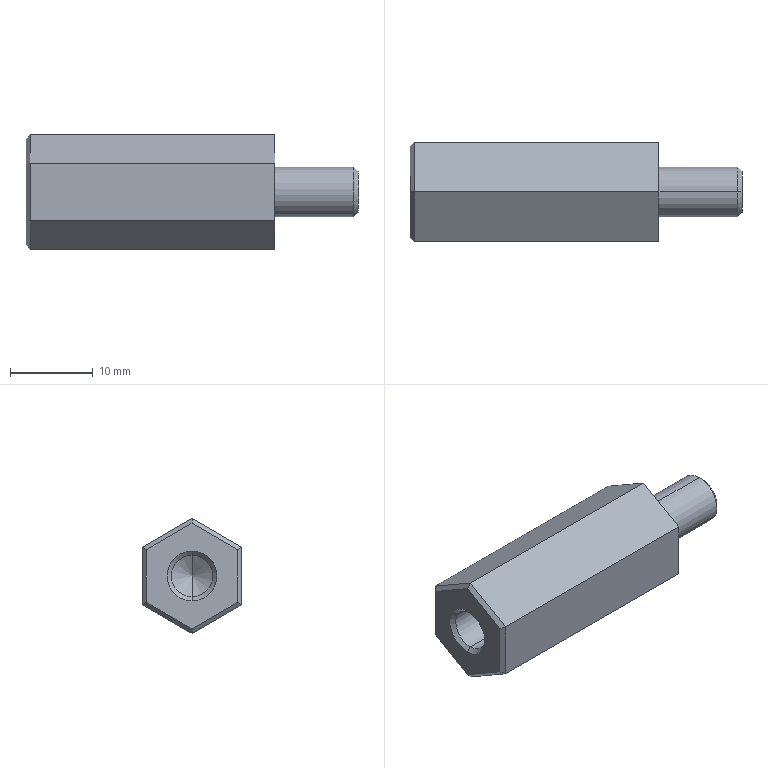Part | SolidWorks | features BaseBody 1 | 1 solid | 25 faces | box 40 x 12 x 13.856 mm | volume 3671 mm3 | plane 15 | cone 6 | cylinder 4 | commonest cylinder face diameters 5 x2 6 x2
STEP:
#1=CARTESIAN_POINT('',(7.747,1875.25,-345.));
#2=VERTEX_POINT('',#1);
#3=CARTESIAN_POINT('',(7.747,1875.25,-351.));
#4=VERTEX_POINT('',#3);
#5=CARTESIAN_POINT('',(7.747,1875.25,-348.));
#6=DIRECTION('',(-1.,0.,0.));
#7=DIRECTION('',(0.,0.,1.));
#8=AXIS2_PLACEMENT_3D('',#5,#6,#7);
#9=CIRCLE('',#8,3.);
#10=EDGE_CURVE('',#2,#4,#9,.T.);
#11=ORIENTED_EDGE('',*,*,#10,.T.);
#12=CARTESIAN_POINT('',(-1.753,1875.25,-351.));
#13=VERTEX_POINT('',#12);
#14=CARTESIAN_POINT('',(8.247,1875.25,-351.));
#15=DIRECTION('',(-1.,0.,0.));
#16=VECTOR('',#15,1000.);
#17=LINE('',#14,#16);
#18=EDGE_CURVE('',#4,#13,#17,.T.);
#19=ORIENTED_EDGE('',*,*,#18,.T.);
#20=CARTESIAN_POINT('',(-1.753,1875.25,-345.));
#21=VERTEX_POINT('',#20);
#22=CARTESIAN_POINT('',(-1.753,1875.25,-348.));
#23=DIRECTION('',(1.,0.,0.));
#24=DIRECTION('',(0.,0.,1.));
#25=AXIS2_PLACEMENT_3D('',#22,#23,#24);
#26=CIRCLE('',#25,3.);
#27=EDGE_CURVE('',#13,#21,#26,.T.);
#28=ORIENTED_EDGE('',*,*,#27,.T.);
#29=CARTESIAN_POINT('',(8.247,1875.25,-345.));
#30=DIRECTION('',(-1.,0.,0.));
#31=VECTOR('',#30,1000.);
#32=LINE('',#29,#31);
#33=EDGE_CURVE('',#2,#21,#32,.T.);
#34=ORIENTED_EDGE('',*,*,#33,.F.);
#35=EDGE_LOOP('',(#11,#19,#28,#34));
#36=FACE_OUTER_BOUND('',#35,.T.);
#37=CARTESIAN_POINT('',(8.247,1875.25,-348.));
#38=DIRECTION('',(-1.,0.,0.));
#39=DIRECTION('',(0.,0.,1.));
#40=AXIS2_PLACEMENT_3D('',#37,#38,#39);
#41=CYLINDRICAL_SURFACE('',#40,3.);
#42=ADVANCED_FACE('',(#36),#41,.T.);
#43=CARTESIAN_POINT('',(8.247,1875.25,-345.5));
#44=VERTEX_POINT('',#43);
#45=CARTESIAN_POINT('',(8.247,1875.25,-350.5));
#46=VERTEX_POINT('',#45);
#47=CARTESIAN_POINT('',(8.247,1875.25,-348.));
#48=DIRECTION('',(-1.,0.,0.));
#49=DIRECTION('',(0.,0.,1.));
#50=AXIS2_PLACEMENT_3D('',#47,#48,#49);
#51=CIRCLE('',#50,2.5);
#52=EDGE_CURVE('',#44,#46,#51,.T.);
#53=ORIENTED_EDGE('',*,*,#52,.T.);
#54=CARTESIAN_POINT('',(7.747,1875.25,-351.));
#55=DIRECTION('',(-0.7071,0.,-0.7071));
#56=VECTOR('',#55,1000.);
#57=LINE('',#54,#56);
#58=EDGE_CURVE('',#46,#4,#57,.T.);
#59=ORIENTED_EDGE('',*,*,#58,.T.);
#60=ORIENTED_EDGE('',*,*,#10,.F.);
#61=CARTESIAN_POINT('',(7.747,1875.25,-345.));
#62=DIRECTION('',(-0.7071,0.,0.7071));
#63=VECTOR('',#62,1000.);
#64=LINE('',#61,#63);
#65=EDGE_CURVE('',#44,#2,#64,.T.);
#66=ORIENTED_EDGE('',*,*,#65,.F.);
#67=EDGE_LOOP('',(#53,#59,#60,#66));
#68=FACE_OUTER_BOUND('',#67,.T.);
#69=CARTESIAN_POINT('',(7.747,1875.25,-348.));
#70=DIRECTION('',(-1.,0.,0.));
#71=DIRECTION('',(0.,0.,1.));
#72=AXIS2_PLACEMENT_3D('',#69,#70,#71);
#73=CONICAL_SURFACE('',#72,3.,0.7854);
#74=ADVANCED_FACE('',(#68),#73,.T.);
#75=CARTESIAN_POINT('',(-31.253,1875.25,-350.5));
#76=VERTEX_POINT('',#75);
#77=CARTESIAN_POINT('',(-31.253,1875.25,-345.5));
#78=VERTEX_POINT('',#77);
#79=CARTESIAN_POINT('',(-31.253,1875.25,-348.));
#80=DIRECTION('',(-1.,0.,0.));
#81=DIRECTION('',(0.,-1.,0.));
#82=AXIS2_PLACEMENT_3D('',#79,#80,#81);
#83=CIRCLE('',#82,2.5);
#84=EDGE_CURVE('',#76,#78,#83,.T.);
#85=ORIENTED_EDGE('',*,*,#84,.F.);
#86=CARTESIAN_POINT('',(-31.753,1875.25,-351.));
#87=VERTEX_POINT('',#86);
#88=CARTESIAN_POINT('',(-31.753,1875.25,-351.));
#89=DIRECTION('',(-0.7071,0.,-0.7071));
#90=VECTOR('',#89,1000.);
#91=LINE('',#88,#90);
#92=EDGE_CURVE('',#76,#87,#91,.T.);
#93=ORIENTED_EDGE('',*,*,#92,.T.);
#94=CARTESIAN_POINT('',(-31.753,1875.25,-345.));
#95=VERTEX_POINT('',#94);
#96=CARTESIAN_POINT('',(-31.753,1875.25,-348.));
#97=DIRECTION('',(1.,0.,0.));
#98=DIRECTION('',(0.,0.,1.));
#99=AXIS2_PLACEMENT_3D('',#96,#97,#98);
#100=CIRCLE('',#99,3.);
#101=EDGE_CURVE('',#95,#87,#100,.T.);
#102=ORIENTED_EDGE('',*,*,#101,.F.);
#103=CARTESIAN_POINT('',(-31.753,1875.25,-345.));
#104=DIRECTION('',(-0.7071,0.,0.7071));
#105=VECTOR('',#104,1000.);
#106=LINE('',#103,#105);
#107=EDGE_CURVE('',#78,#95,#106,.T.);
#108=ORIENTED_EDGE('',*,*,#107,.F.);
#109=EDGE_LOOP('',(#85,#93,#102,#108));
#110=FACE_OUTER_BOUND('',#109,.T.);
#111=CARTESIAN_POINT('',(-31.753,1875.25,-348.));
#112=DIRECTION('',(-1.,0.,0.));
#113=DIRECTION('',(0.,0.,1.));
#114=AXIS2_PLACEMENT_3D('',#111,#112,#113);
#115=CONICAL_SURFACE('',#114,3.,0.7854);
#116=ADVANCED_FACE('',(#110),#115,.F.);
#117=CARTESIAN_POINT('',(-14.753,1875.25,-350.5));
#118=VERTEX_POINT('',#117);
#119=CARTESIAN_POINT('',(-14.753,1875.25,-345.5));
#120=VERTEX_POINT('',#119);
#121=CARTESIAN_POINT('',(-14.753,1875.25,-348.));
#122=DIRECTION('',(-1.,0.,0.));
#123=DIRECTION('',(0.,0.,1.));
#124=AXIS2_PLACEMENT_3D('',#121,#122,#123);
#125=CIRCLE('',#124,2.5);
#126=EDGE_CURVE('',#118,#120,#125,.T.);
#127=ORIENTED_EDGE('',*,*,#126,.F.);
#128=CARTESIAN_POINT('',(-31.753,1875.25,-350.5));
#129=DIRECTION('',(-1.,0.,0.));
#130=VECTOR('',#129,1000.);
#131=LINE('',#128,#130);
#132=EDGE_CURVE('',#118,#76,#131,.T.);
#133=ORIENTED_EDGE('',*,*,#132,.T.);
#134=ORIENTED_EDGE('',*,*,#84,.T.);
#135=CARTESIAN_POINT('',(-31.753,1875.25,-345.5));
#136=DIRECTION('',(-1.,0.,0.));
#137=VECTOR('',#136,1000.);
#138=LINE('',#135,#137);
#139=EDGE_CURVE('',#120,#78,#138,.T.);
#140=ORIENTED_EDGE('',*,*,#139,.F.);
#141=EDGE_LOOP('',(#127,#133,#134,#140));
#142=FACE_OUTER_BOUND('',#141,.T.);
#143=CARTESIAN_POINT('',(-31.753,1875.25,-348.));
#144=DIRECTION('',(-1.,0.,0.));
#145=DIRECTION('',(0.,0.,1.));
#146=AXIS2_PLACEMENT_3D('',#143,#144,#145);
#147=CYLINDRICAL_SURFACE('',#146,2.5);
#148=ADVANCED_FACE('',(#142),#147,.F.);
#149=CARTESIAN_POINT('',(-13.251,1875.25,-348.));
#150=VERTEX_POINT('',#149);
#151=CARTESIAN_POINT('',(-14.753,1875.25,-345.5));
#152=DIRECTION('',(-0.515,0.,0.8572));
#153=VECTOR('',#152,1000.);
#154=LINE('',#151,#153);
#155=EDGE_CURVE('',#150,#120,#154,.T.);
#156=ORIENTED_EDGE('',*,*,#155,.F.);
#157=CARTESIAN_POINT('',(-14.753,1875.25,-350.5));
#158=DIRECTION('',(-0.515,0.,-0.8572));
#159=VECTOR('',#158,1000.);
#160=LINE('',#157,#159);
#161=EDGE_CURVE('',#150,#118,#160,.T.);
#162=ORIENTED_EDGE('',*,*,#161,.T.);
#163=ORIENTED_EDGE('',*,*,#126,.T.);
#164=EDGE_LOOP('',(#156,#162,#163));
#165=FACE_OUTER_BOUND('',#164,.T.);
#166=CARTESIAN_POINT('',(-14.753,1875.25,-348.));
#167=DIRECTION('',(-1.,0.,0.));
#168=DIRECTION('',(0.,0.,1.));
#169=AXIS2_PLACEMENT_3D('',#166,#167,#168);
#170=CONICAL_SURFACE('',#169,2.5,1.03);
#171=ADVANCED_FACE('',(#165),#170,.F.);
#172=CARTESIAN_POINT('',(-1.753,1875.25,-354.928));
#173=VERTEX_POINT('',#172);
#174=CARTESIAN_POINT('',(-1.753,1869.25,-351.464));
#175=VERTEX_POINT('',#174);
#176=CARTESIAN_POINT('',(-1.753,1875.25,-354.928));
#177=DIRECTION('',(0.,-0.866,0.5));
#178=VECTOR('',#177,1000.);
#179=LINE('',#176,#178);
#180=EDGE_CURVE('',#173,#175,#179,.T.);
#181=ORIENTED_EDGE('',*,*,#180,.T.);
#182=CARTESIAN_POINT('',(-31.253,1869.25,-351.464));
#183=VERTEX_POINT('',#182);
#184=CARTESIAN_POINT('',(-1.753,1869.25,-351.464));
#185=DIRECTION('',(-1.,0.,0.));
#186=VECTOR('',#185,1000.);
#187=LINE('',#184,#186);
#188=EDGE_CURVE('',#175,#183,#187,.T.);
#189=ORIENTED_EDGE('',*,*,#188,.T.);
#190=CARTESIAN_POINT('',(-31.253,1875.25,-354.928));
#191=VERTEX_POINT('',#190);
#192=CARTESIAN_POINT('',(-31.253,1875.25,-354.928));
#193=DIRECTION('',(0.,0.866,-0.5));
#194=VECTOR('',#193,1000.);
#195=LINE('',#192,#194);
#196=EDGE_CURVE('',#183,#191,#195,.T.);
#197=ORIENTED_EDGE('',*,*,#196,.T.);
#198=CARTESIAN_POINT('',(-1.753,1875.25,-354.928));
#199=DIRECTION('',(1.,0.,0.));
#200=VECTOR('',#199,1000.);
#201=LINE('',#198,#200);
#202=EDGE_CURVE('',#191,#173,#201,.T.);
#203=ORIENTED_EDGE('',*,*,#202,.T.);
#204=EDGE_LOOP('',(#181,#189,#197,#203));
#205=FACE_OUTER_BOUND('',#204,.T.);
#206=CARTESIAN_POINT('',(-1.753,1875.25,-354.928));
#207=DIRECTION('',(0.,-0.5,-0.866));
#208=DIRECTION('',(0.,0.866,-0.5));
#209=AXIS2_PLACEMENT_3D('',#206,#207,#208);
#210=PLANE('',#209);
#211=ADVANCED_FACE('',(#205),#210,.T.);
#212=CARTESIAN_POINT('',(-1.753,1869.25,-344.536));
#213=VERTEX_POINT('',#212);
#214=CARTESIAN_POINT('',(-1.753,1869.25,-351.464));
#215=DIRECTION('',(0.,0.,1.));
#216=VECTOR('',#215,1000.);
#217=LINE('',#214,#216);
#218=EDGE_CURVE('',#175,#213,#217,.T.);
#219=ORIENTED_EDGE('',*,*,#218,.T.);
#220=CARTESIAN_POINT('',(-31.253,1869.25,-344.536));
#221=VERTEX_POINT('',#220);
#222=CARTESIAN_POINT('',(-1.753,1869.25,-344.536));
#223=DIRECTION('',(-1.,0.,0.));
#224=VECTOR('',#223,1000.);
#225=LINE('',#222,#224);
#226=EDGE_CURVE('',#213,#221,#225,.T.);
#227=ORIENTED_EDGE('',*,*,#226,.T.);
#228=CARTESIAN_POINT('',(-31.253,1869.25,-351.464));
#229=DIRECTION('',(0.,0.,-1.));
#230=VECTOR('',#229,1000.);
#231=LINE('',#228,#230);
#232=EDGE_CURVE('',#221,#183,#231,.T.);
#233=ORIENTED_EDGE('',*,*,#232,.T.);
#234=ORIENTED_EDGE('',*,*,#188,.F.);
#235=EDGE_LOOP('',(#219,#227,#233,#234));
#236=FACE_OUTER_BOUND('',#235,.T.);
#237=CARTESIAN_POINT('',(-1.753,1869.25,-351.464));
#238=DIRECTION('',(0.,-1.,0.));
#239=DIRECTION('',(0.,0.,-1.));
#240=AXIS2_PLACEMENT_3D('',#237,#238,#239);
#241=PLANE('',#240);
#242=ADVANCED_FACE('',(#236),#241,.T.);
#243=CARTESIAN_POINT('',(-1.753,1875.25,-348.));
#244=DIRECTION('',(1.,0.,0.));
#245=DIRECTION('',(0.,0.,1.));
#246=AXIS2_PLACEMENT_3D('',#243,#244,#245);
#247=CIRCLE('',#246,3.);
#248=EDGE_CURVE('',#21,#13,#247,.T.);
#249=ORIENTED_EDGE('',*,*,#248,.F.);
#250=ORIENTED_EDGE('',*,*,#27,.F.);
#251=EDGE_LOOP('',(#249,#250));
#252=FACE_BOUND('',#251,.T.);
#253=CARTESIAN_POINT('',(-1.753,1881.25,-344.536));
#254=VERTEX_POINT('',#253);
#255=CARTESIAN_POINT('',(-1.753,1881.25,-351.464));
#256=VERTEX_POINT('',#255);
#257=CARTESIAN_POINT('',(-1.753,1881.25,-348.));
#258=DIRECTION('',(0.,0.,-1.));
#259=VECTOR('',#258,1000.);
#260=LINE('',#257,#259);
#261=EDGE_CURVE('',#254,#256,#260,.T.);
#262=ORIENTED_EDGE('',*,*,#261,.F.);
#263=CARTESIAN_POINT('',(-1.753,1875.25,-341.072));
#264=VERTEX_POINT('',#263);
#265=CARTESIAN_POINT('',(-1.753,1875.25,-341.072));
#266=DIRECTION('',(0.,0.866,-0.5));
#267=VECTOR('',#266,1000.);
#268=LINE('',#265,#267);
#269=EDGE_CURVE('',#264,#254,#268,.T.);
#270=ORIENTED_EDGE('',*,*,#269,.F.);
#271=CARTESIAN_POINT('',(-1.753,1869.25,-344.536));
#272=DIRECTION('',(0.,0.866,0.5));
#273=VECTOR('',#272,1000.);
#274=LINE('',#271,#273);
#275=EDGE_CURVE('',#213,#264,#274,.T.);
#276=ORIENTED_EDGE('',*,*,#275,.F.);
#277=ORIENTED_EDGE('',*,*,#218,.F.);
#278=ORIENTED_EDGE('',*,*,#180,.F.);
#279=CARTESIAN_POINT('',(-1.753,1881.25,-351.464));
#280=DIRECTION('',(0.,-0.866,-0.5));
#281=VECTOR('',#280,1000.);
#282=LINE('',#279,#281);
#283=EDGE_CURVE('',#256,#173,#282,.T.);
#284=ORIENTED_EDGE('',*,*,#283,.F.);
#285=EDGE_LOOP('',(#262,#270,#276,#277,#278,#284));
#286=FACE_OUTER_BOUND('',#285,.T.);
#287=CARTESIAN_POINT('',(-1.753,1875.25,-348.));
#288=DIRECTION('',(-1.,0.,0.));
#289=DIRECTION('',(0.,0.,1.));
#290=AXIS2_PLACEMENT_3D('',#287,#288,#289);
#291=PLANE('',#290);
#292=ADVANCED_FACE('',(#252,#286),#291,.F.);
#293=ORIENTED_EDGE('',*,*,#283,.T.);
#294=ORIENTED_EDGE('',*,*,#202,.F.);
#295=CARTESIAN_POINT('',(-31.253,1881.25,-351.464));
#296=VERTEX_POINT('',#295);
#297=CARTESIAN_POINT('',(-31.253,1881.25,-351.464));
#298=DIRECTION('',(0.,0.866,0.5));
#299=VECTOR('',#298,1000.);
#300=LINE('',#297,#299);
#301=EDGE_CURVE('',#191,#296,#300,.T.);
#302=ORIENTED_EDGE('',*,*,#301,.T.);
#303=CARTESIAN_POINT('',(-1.753,1881.25,-351.464));
#304=DIRECTION('',(1.,0.,0.));
#305=VECTOR('',#304,1000.);
#306=LINE('',#303,#305);
#307=EDGE_CURVE('',#296,#256,#306,.T.);
#308=ORIENTED_EDGE('',*,*,#307,.T.);
#309=EDGE_LOOP('',(#293,#294,#302,#308));
#310=FACE_OUTER_BOUND('',#309,.T.);
#311=CARTESIAN_POINT('',(-1.753,1881.25,-351.464));
#312=DIRECTION('',(0.,0.5,-0.866));
#313=DIRECTION('',(0.,0.866,0.5));
#314=AXIS2_PLACEMENT_3D('',#311,#312,#313);
#315=PLANE('',#314);
#316=ADVANCED_FACE('',(#310),#315,.T.);
#317=CARTESIAN_POINT('',(-31.753,1875.25,-354.351));
#318=VERTEX_POINT('',#317);
#319=CARTESIAN_POINT('',(-32.539,1875.25,-353.444));
#320=DIRECTION('',(-0.6547,0.,0.7559));
#321=VECTOR('',#320,1000.);
#322=LINE('',#319,#321);
#323=EDGE_CURVE('',#191,#318,#322,.T.);
#324=ORIENTED_EDGE('',*,*,#323,.F.);
#325=ORIENTED_EDGE('',*,*,#196,.F.);
#326=CARTESIAN_POINT('',(-31.753,1869.75,-351.175));
#327=VERTEX_POINT('',#326);
#328=CARTESIAN_POINT('',(-31.753,1869.75,-351.175));
#329=DIRECTION('',(0.6547,-0.6547,-0.378));
#330=VECTOR('',#329,1000.);
#331=LINE('',#328,#330);
#332=EDGE_CURVE('',#327,#183,#331,.T.);
#333=ORIENTED_EDGE('',*,*,#332,.F.);
#334=CARTESIAN_POINT('',(-31.753,1875.25,-354.351));
#335=DIRECTION('',(0.,-0.866,0.5));
#336=VECTOR('',#335,1000.);
#337=LINE('',#334,#336);
#338=EDGE_CURVE('',#318,#327,#337,.T.);
#339=ORIENTED_EDGE('',*,*,#338,.F.);
#340=EDGE_LOOP('',(#324,#325,#333,#339));
#341=FACE_OUTER_BOUND('',#340,.T.);
#342=CARTESIAN_POINT('',(-31.753,1872.5,-352.763));
#343=DIRECTION('',(0.7071,0.3536,0.6124));
#344=DIRECTION('',(0.6547,0.,-0.7559));
#345=AXIS2_PLACEMENT_3D('',#342,#343,#344);
#346=PLANE('',#345);
#347=ADVANCED_FACE('',(#341),#346,.F.);
#348=ORIENTED_EDGE('',*,*,#275,.T.);
#349=CARTESIAN_POINT('',(-31.253,1875.25,-341.072));
#350=VERTEX_POINT('',#349);
#351=CARTESIAN_POINT('',(-1.753,1875.25,-341.072));
#352=DIRECTION('',(-1.,0.,0.));
#353=VECTOR('',#352,1000.);
#354=LINE('',#351,#353);
#355=EDGE_CURVE('',#264,#350,#354,.T.);
#356=ORIENTED_EDGE('',*,*,#355,.T.);
#357=CARTESIAN_POINT('',(-31.253,1869.25,-344.536));
#358=DIRECTION('',(0.,-0.866,-0.5));
#359=VECTOR('',#358,1000.);
#360=LINE('',#357,#359);
#361=EDGE_CURVE('',#350,#221,#360,.T.);
#362=ORIENTED_EDGE('',*,*,#361,.T.);
#363=ORIENTED_EDGE('',*,*,#226,.F.);
#364=EDGE_LOOP('',(#348,#356,#362,#363));
#365=FACE_OUTER_BOUND('',#364,.T.);
#366=CARTESIAN_POINT('',(-1.753,1869.25,-344.536));
#367=DIRECTION('',(0.,-0.5,0.866));
#368=DIRECTION('',(0.,-0.866,-0.5));
#369=AXIS2_PLACEMENT_3D('',#366,#367,#368);
#370=PLANE('',#369);
#371=ADVANCED_FACE('',(#365),#370,.T.);
#372=ORIENTED_EDGE('',*,*,#332,.T.);
#373=ORIENTED_EDGE('',*,*,#232,.F.);
#374=CARTESIAN_POINT('',(-31.753,1869.75,-344.825));
#375=VERTEX_POINT('',#374);
#376=CARTESIAN_POINT('',(-31.753,1869.75,-344.825));
#377=DIRECTION('',(0.6547,-0.6547,0.378));
#378=VECTOR('',#377,1000.);
#379=LINE('',#376,#378);
#380=EDGE_CURVE('',#375,#221,#379,.T.);
#381=ORIENTED_EDGE('',*,*,#380,.F.);
#382=CARTESIAN_POINT('',(-31.753,1869.75,-348.));
#383=DIRECTION('',(0.,0.,1.));
#384=VECTOR('',#383,1000.);
#385=LINE('',#382,#384);
#386=EDGE_CURVE('',#327,#375,#385,.T.);
#387=ORIENTED_EDGE('',*,*,#386,.F.);
#388=EDGE_LOOP('',(#372,#373,#381,#387));
#389=FACE_OUTER_BOUND('',#388,.T.);
#390=CARTESIAN_POINT('',(-31.753,1869.75,-348.));
#391=DIRECTION('',(0.7071,0.7071,0.));
#392=DIRECTION('',(-0.7071,0.7071,0.));
#393=AXIS2_PLACEMENT_3D('',#390,#391,#392);
#394=PLANE('',#393);
#395=ADVANCED_FACE('',(#389),#394,.F.);
#396=ORIENTED_EDGE('',*,*,#18,.F.);
#397=CARTESIAN_POINT('',(7.747,1875.25,-348.));
#398=DIRECTION('',(-1.,0.,0.));
#399=DIRECTION('',(0.,0.,1.));
#400=AXIS2_PLACEMENT_3D('',#397,#398,#399);
#401=CIRCLE('',#400,3.);
#402=EDGE_CURVE('',#4,#2,#401,.T.);
#403=ORIENTED_EDGE('',*,*,#402,.T.);
#404=ORIENTED_EDGE('',*,*,#33,.T.);
#405=ORIENTED_EDGE('',*,*,#248,.T.);
#406=EDGE_LOOP('',(#396,#403,#404,#405));
#407=FACE_OUTER_BOUND('',#406,.T.);
#408=CARTESIAN_POINT('',(8.247,1875.25,-348.));
#409=DIRECTION('',(-1.,0.,0.));
#410=DIRECTION('',(0.,0.,1.));
#411=AXIS2_PLACEMENT_3D('',#408,#409,#410);
#412=CYLINDRICAL_SURFACE('',#411,3.);
#413=ADVANCED_FACE('',(#407),#412,.T.);
#414=ORIENTED_EDGE('',*,*,#261,.T.);
#415=ORIENTED_EDGE('',*,*,#307,.F.);
#416=CARTESIAN_POINT('',(-31.253,1881.25,-344.536));
#417=VERTEX_POINT('',#416);
#418=CARTESIAN_POINT('',(-31.253,1881.25,-344.536));
#419=DIRECTION('',(0.,0.,1.));
#420=VECTOR('',#419,1000.);
#421=LINE('',#418,#420);
#422=EDGE_CURVE('',#296,#417,#421,.T.);
#423=ORIENTED_EDGE('',*,*,#422,.T.);
#424=CARTESIAN_POINT('',(-1.753,1881.25,-344.536));
#425=DIRECTION('',(1.,0.,0.));
#426=VECTOR('',#425,1000.);
#427=LINE('',#424,#426);
#428=EDGE_CURVE('',#417,#254,#427,.T.);
#429=ORIENTED_EDGE('',*,*,#428,.T.);
#430=EDGE_LOOP('',(#414,#415,#423,#429));
#431=FACE_OUTER_BOUND('',#430,.T.);
#432=CARTESIAN_POINT('',(-1.753,1881.25,-344.536));
#433=DIRECTION('',(0.,1.,0.));
#434=DIRECTION('',(0.,0.,1.));
#435=AXIS2_PLACEMENT_3D('',#432,#433,#434);
#436=PLANE('',#435);
#437=ADVANCED_FACE('',(#431),#436,.T.);
#438=ORIENTED_EDGE('',*,*,#269,.T.);
#439=ORIENTED_EDGE('',*,*,#428,.F.);
#440=CARTESIAN_POINT('',(-31.253,1875.25,-341.072));
#441=DIRECTION('',(0.,-0.866,0.5));
#442=VECTOR('',#441,1000.);
#443=LINE('',#440,#442);
#444=EDGE_CURVE('',#417,#350,#443,.T.);
#445=ORIENTED_EDGE('',*,*,#444,.T.);
#446=ORIENTED_EDGE('',*,*,#355,.F.);
#447=EDGE_LOOP('',(#438,#439,#445,#446));
#448=FACE_OUTER_BOUND('',#447,.T.);
#449=CARTESIAN_POINT('',(-1.753,1875.25,-341.072));
#450=DIRECTION('',(0.,0.5,0.866));
#451=DIRECTION('',(0.,-0.866,0.5));
#452=AXIS2_PLACEMENT_3D('',#449,#450,#451);
#453=PLANE('',#452);
#454=ADVANCED_FACE('',(#448),#453,.T.);
#455=ORIENTED_EDGE('',*,*,#323,.T.);
#456=CARTESIAN_POINT('',(-31.753,1880.75,-351.175));
#457=VERTEX_POINT('',#456);
#458=CARTESIAN_POINT('',(-31.753,1880.75,-351.175));
#459=DIRECTION('',(0.,-0.866,-0.5));
#460=VECTOR('',#459,1000.);
#461=LINE('',#458,#460);
#462=EDGE_CURVE('',#457,#318,#461,.T.);
#463=ORIENTED_EDGE('',*,*,#462,.F.);
#464=CARTESIAN_POINT('',(-31.253,1881.25,-351.464));
#465=DIRECTION('',(-0.6547,-0.6547,0.378));
#466=VECTOR('',#465,1000.);
#467=LINE('',#464,#466);
#468=EDGE_CURVE('',#296,#457,#467,.T.);
#469=ORIENTED_EDGE('',*,*,#468,.F.);
#470=ORIENTED_EDGE('',*,*,#301,.F.);
#471=EDGE_LOOP('',(#455,#463,#469,#470));
#472=FACE_OUTER_BOUND('',#471,.T.);
#473=CARTESIAN_POINT('',(-31.753,1878.,-352.763));
#474=DIRECTION('',(0.7071,-0.3536,0.6124));
#475=DIRECTION('',(0.6547,0.,-0.7559));
#476=AXIS2_PLACEMENT_3D('',#473,#474,#475);
#477=PLANE('',#476);
#478=ADVANCED_FACE('',(#472),#477,.F.);
#479=ORIENTED_EDGE('',*,*,#101,.T.);
#480=CARTESIAN_POINT('',(-31.753,1875.25,-348.));
#481=DIRECTION('',(1.,0.,0.));
#482=DIRECTION('',(0.,0.,1.));
#483=AXIS2_PLACEMENT_3D('',#480,#481,#482);
#484=CIRCLE('',#483,3.);
#485=EDGE_CURVE('',#87,#95,#484,.T.);
#486=ORIENTED_EDGE('',*,*,#485,.T.);
#487=EDGE_LOOP('',(#479,#486));
#488=FACE_BOUND('',#487,.T.);
#489=CARTESIAN_POINT('',(-31.753,1875.25,-341.649));
#490=VERTEX_POINT('',#489);
#491=CARTESIAN_POINT('',(-31.753,1880.75,-344.825));
#492=VERTEX_POINT('',#491);
#493=CARTESIAN_POINT('',(-31.753,1875.25,-341.649));
#494=DIRECTION('',(0.,0.866,-0.5));
#495=VECTOR('',#494,1000.);
#496=LINE('',#493,#495);
#497=EDGE_CURVE('',#490,#492,#496,.T.);
#498=ORIENTED_EDGE('',*,*,#497,.T.);
#499=CARTESIAN_POINT('',(-31.753,1880.75,-348.));
#500=DIRECTION('',(0.,0.,-1.));
#501=VECTOR('',#500,1000.);
#502=LINE('',#499,#501);
#503=EDGE_CURVE('',#492,#457,#502,.T.);
#504=ORIENTED_EDGE('',*,*,#503,.T.);
#505=ORIENTED_EDGE('',*,*,#462,.T.);
#506=ORIENTED_EDGE('',*,*,#338,.T.);
#507=ORIENTED_EDGE('',*,*,#386,.T.);
#508=CARTESIAN_POINT('',(-31.753,1869.75,-344.825));
#509=DIRECTION('',(0.,0.866,0.5));
#510=VECTOR('',#509,1000.);
#511=LINE('',#508,#510);
#512=EDGE_CURVE('',#375,#490,#511,.T.);
#513=ORIENTED_EDGE('',*,*,#512,.T.);
#514=EDGE_LOOP('',(#498,#504,#505,#506,#507,#513));
#515=FACE_OUTER_BOUND('',#514,.T.);
#516=CARTESIAN_POINT('',(-31.753,1875.25,-348.));
#517=DIRECTION('',(-1.,0.,0.));
#518=DIRECTION('',(0.,0.,1.));
#519=AXIS2_PLACEMENT_3D('',#516,#517,#518);
#520=PLANE('',#519);
#521=ADVANCED_FACE('',(#488,#515),#520,.T.);
#522=CARTESIAN_POINT('',(-32.539,1875.25,-342.556));
#523=DIRECTION('',(0.6547,0.,0.7559));
#524=VECTOR('',#523,1000.);
#525=LINE('',#522,#524);
#526=EDGE_CURVE('',#490,#350,#525,.T.);
#527=ORIENTED_EDGE('',*,*,#526,.F.);
#528=ORIENTED_EDGE('',*,*,#512,.F.);
#529=ORIENTED_EDGE('',*,*,#380,.T.);
#530=ORIENTED_EDGE('',*,*,#361,.F.);
#531=EDGE_LOOP('',(#527,#528,#529,#530));
#532=FACE_OUTER_BOUND('',#531,.T.);
#533=CARTESIAN_POINT('',(-31.753,1872.5,-343.237));
#534=DIRECTION('',(0.7071,0.3536,-0.6124));
#535=DIRECTION('',(-0.6547,0.,-0.7559));
#536=AXIS2_PLACEMENT_3D('',#533,#534,#535);
#537=PLANE('',#536);
#538=ADVANCED_FACE('',(#532),#537,.F.);
#539=ORIENTED_EDGE('',*,*,#58,.F.);
#540=CARTESIAN_POINT('',(8.247,1875.25,-348.));
#541=DIRECTION('',(-1.,0.,0.));
#542=DIRECTION('',(0.,0.,1.));
#543=AXIS2_PLACEMENT_3D('',#540,#541,#542);
#544=CIRCLE('',#543,2.5);
#545=EDGE_CURVE('',#46,#44,#544,.T.);
#546=ORIENTED_EDGE('',*,*,#545,.T.);
#547=ORIENTED_EDGE('',*,*,#65,.T.);
#548=ORIENTED_EDGE('',*,*,#402,.F.);
#549=EDGE_LOOP('',(#539,#546,#547,#548));
#550=FACE_OUTER_BOUND('',#549,.T.);
#551=CARTESIAN_POINT('',(7.747,1875.25,-348.));
#552=DIRECTION('',(-1.,0.,0.));
#553=DIRECTION('',(0.,0.,1.));
#554=AXIS2_PLACEMENT_3D('',#551,#552,#553);
#555=CONICAL_SURFACE('',#554,3.,0.7854);
#556=ADVANCED_FACE('',(#550),#555,.T.);
#557=ORIENTED_EDGE('',*,*,#468,.T.);
#558=ORIENTED_EDGE('',*,*,#503,.F.);
#559=CARTESIAN_POINT('',(-31.253,1881.25,-344.536));
#560=DIRECTION('',(-0.6547,-0.6547,-0.378));
#561=VECTOR('',#560,1000.);
#562=LINE('',#559,#561);
#563=EDGE_CURVE('',#417,#492,#562,.T.);
#564=ORIENTED_EDGE('',*,*,#563,.F.);
#565=ORIENTED_EDGE('',*,*,#422,.F.);
#566=EDGE_LOOP('',(#557,#558,#564,#565));
#567=FACE_OUTER_BOUND('',#566,.T.);
#568=CARTESIAN_POINT('',(-31.753,1880.75,-348.));
#569=DIRECTION('',(0.7071,-0.7071,0.));
#570=DIRECTION('',(0.7071,0.7071,0.));
#571=AXIS2_PLACEMENT_3D('',#568,#569,#570);
#572=PLANE('',#571);
#573=ADVANCED_FACE('',(#567),#572,.F.);
#574=ORIENTED_EDGE('',*,*,#563,.T.);
#575=ORIENTED_EDGE('',*,*,#497,.F.);
#576=ORIENTED_EDGE('',*,*,#526,.T.);
#577=ORIENTED_EDGE('',*,*,#444,.F.);
#578=EDGE_LOOP('',(#574,#575,#576,#577));
#579=FACE_OUTER_BOUND('',#578,.T.);
#580=CARTESIAN_POINT('',(-31.753,1878.,-343.237));
#581=DIRECTION('',(0.7071,-0.3536,-0.6124));
#582=DIRECTION('',(-0.6547,0.,-0.7559));
#583=AXIS2_PLACEMENT_3D('',#580,#581,#582);
#584=PLANE('',#583);
#585=ADVANCED_FACE('',(#579),#584,.F.);
#586=ORIENTED_EDGE('',*,*,#92,.F.);
#587=CARTESIAN_POINT('',(-31.253,1875.25,-348.));
#588=DIRECTION('',(-1.,0.,0.));
#589=DIRECTION('',(0.,-1.,0.));
#590=AXIS2_PLACEMENT_3D('',#587,#588,#589);
#591=CIRCLE('',#590,2.5);
#592=EDGE_CURVE('',#78,#76,#591,.T.);
#593=ORIENTED_EDGE('',*,*,#592,.F.);
#594=ORIENTED_EDGE('',*,*,#107,.T.);
#595=ORIENTED_EDGE('',*,*,#485,.F.);
#596=EDGE_LOOP('',(#586,#593,#594,#595));
#597=FACE_OUTER_BOUND('',#596,.T.);
#598=CARTESIAN_POINT('',(-31.753,1875.25,-348.));
#599=DIRECTION('',(-1.,0.,0.));
#600=DIRECTION('',(0.,0.,1.));
#601=AXIS2_PLACEMENT_3D('',#598,#599,#600);
#602=CONICAL_SURFACE('',#601,3.,0.7854);
#603=ADVANCED_FACE('',(#597),#602,.F.);
#604=ORIENTED_EDGE('',*,*,#52,.F.);
#605=ORIENTED_EDGE('',*,*,#545,.F.);
#606=EDGE_LOOP('',(#604,#605));
#607=FACE_OUTER_BOUND('',#606,.T.);
#608=CARTESIAN_POINT('',(8.247,1875.25,-348.));
#609=DIRECTION('',(1.,0.,0.));
#610=DIRECTION('',(0.,0.,-1.));
#611=AXIS2_PLACEMENT_3D('',#608,#609,#610);
#612=PLANE('',#611);
#613=ADVANCED_FACE('',(#607),#612,.T.);
#614=ORIENTED_EDGE('',*,*,#132,.F.);
#615=CARTESIAN_POINT('',(-14.753,1875.25,-348.));
#616=DIRECTION('',(-1.,0.,0.));
#617=DIRECTION('',(0.,0.,1.));
#618=AXIS2_PLACEMENT_3D('',#615,#616,#617);
#619=CIRCLE('',#618,2.5);
#620=EDGE_CURVE('',#120,#118,#619,.T.);
#621=ORIENTED_EDGE('',*,*,#620,.F.);
#622=ORIENTED_EDGE('',*,*,#139,.T.);
#623=ORIENTED_EDGE('',*,*,#592,.T.);
#624=EDGE_LOOP('',(#614,#621,#622,#623));
#625=FACE_OUTER_BOUND('',#624,.T.);
#626=CARTESIAN_POINT('',(-31.753,1875.25,-348.));
#627=DIRECTION('',(-1.,0.,0.));
#628=DIRECTION('',(0.,0.,1.));
#629=AXIS2_PLACEMENT_3D('',#626,#627,#628);
#630=CYLINDRICAL_SURFACE('',#629,2.5);
#631=ADVANCED_FACE('',(#625),#630,.F.);
#632=ORIENTED_EDGE('',*,*,#161,.F.);
#633=ORIENTED_EDGE('',*,*,#155,.T.);
#634=ORIENTED_EDGE('',*,*,#620,.T.);
#635=EDGE_LOOP('',(#632,#633,#634));
#636=FACE_OUTER_BOUND('',#635,.T.);
#637=CARTESIAN_POINT('',(-14.753,1875.25,-348.));
#638=DIRECTION('',(-1.,0.,0.));
#639=DIRECTION('',(0.,0.,1.));
#640=AXIS2_PLACEMENT_3D('',#637,#638,#639);
#641=CONICAL_SURFACE('',#640,2.5,1.03);
#642=ADVANCED_FACE('',(#636),#641,.F.);
#643=CLOSED_SHELL('',(#42,#74,#116,#148,#171,#211,#242,#292,#316,#347,#371,#395,#413,#437,#454,#478,#521,#538,#556,#573,#585,#603,#613,#631,#642));
#644=MANIFOLD_SOLID_BREP('',#643);
#645=CARTESIAN_POINT('',(0.,0.,0.));
#646=DIRECTION('',(0.,0.,1.));
#647=DIRECTION('',(1.,0.,0.));
#648=AXIS2_PLACEMENT_3D('',#645,#646,#647);
#649=(LENGTH_UNIT()NAMED_UNIT(*)SI_UNIT(.MILLI.,.METRE.));
#650=UNCERTAINTY_MEASURE_WITH_UNIT(LENGTH_MEASURE(0.00001),#649,'','');
#651=(NAMED_UNIT(*)PLANE_ANGLE_UNIT()SI_UNIT($,.RADIAN.));
#652=(NAMED_UNIT(*)SI_UNIT($,.STERADIAN.)SOLID_ANGLE_UNIT());
#653=(GEOMETRIC_REPRESENTATION_CONTEXT(3)GLOBAL_UNCERTAINTY_ASSIGNED_CONTEXT((#650))GLOBAL_UNIT_ASSIGNED_CONTEXT((#649,#651,#652))REPRESENTATION_CONTEXT('',''));
#654=ADVANCED_BREP_SHAPE_REPRESENTATION('',(#644,#648),#653);